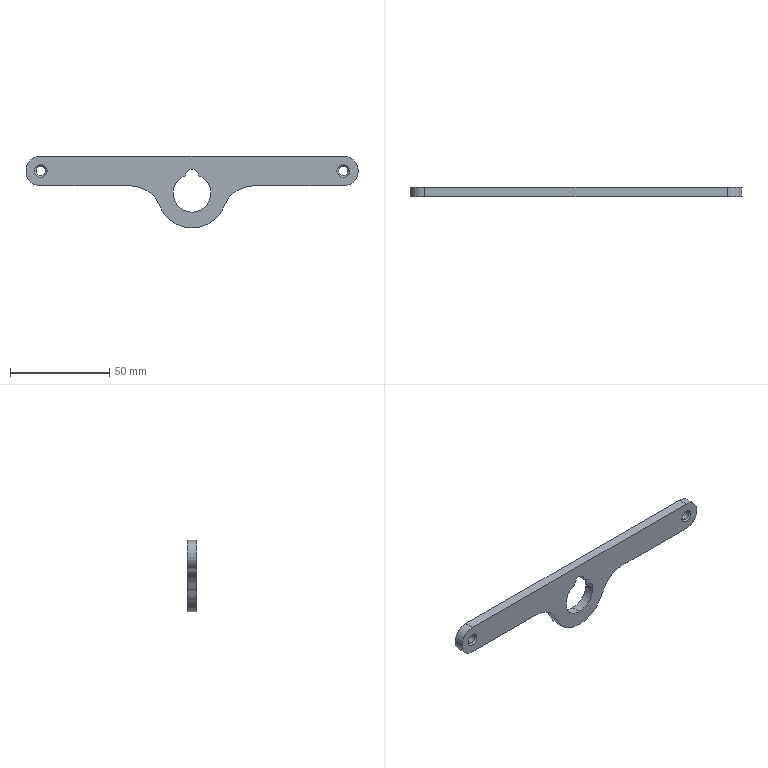Part | SolidWorks | features Chamfer 1, Extrusion 1 | 1 solid | 26 faces | box 167.386 x 4.826 x 36.182 mm | volume 13483 mm3 | cylinder 13 | cone 8 | plane 5 | commonest cylinder face diameters 4.826 x4 14.986 x2 19.025 x2 31.75 x2 34.9 x2 6.35 x1
STEP:
#1=CARTESIAN_POINT('',(-3.,0.065,0.3475));
#2=VERTEX_POINT('',#1);
#3=CARTESIAN_POINT('',(-3.,0.065,0.5375));
#4=VERTEX_POINT('',#3);
#5=CARTESIAN_POINT('',(-3.,0.065,0.4425));
#6=DIRECTION('',(0.,1.,0.));
#7=DIRECTION('',(0.,0.,1.));
#8=AXIS2_PLACEMENT_3D('',#5,#6,#7);
#9=CIRCLE('',#8,0.095);
#10=EDGE_CURVE('',#2,#4,#9,.T.);
#11=ORIENTED_EDGE('',*,*,#10,.F.);
#12=CARTESIAN_POINT('',(-3.,0.095,0.3175));
#13=VERTEX_POINT('',#12);
#14=CARTESIAN_POINT('',(-3.,0.065,0.3475));
#15=DIRECTION('',(0.,0.7071,-0.7071));
#16=VECTOR('',#15,39.37);
#17=LINE('',#14,#16);
#18=EDGE_CURVE('',#2,#13,#17,.T.);
#19=ORIENTED_EDGE('',*,*,#18,.T.);
#20=CARTESIAN_POINT('',(-3.,0.095,0.5675));
#21=VERTEX_POINT('',#20);
#22=CARTESIAN_POINT('',(-3.,0.095,0.4425));
#23=DIRECTION('',(0.,-1.,0.));
#24=DIRECTION('',(0.,0.,1.));
#25=AXIS2_PLACEMENT_3D('',#22,#23,#24);
#26=CIRCLE('',#25,0.125);
#27=EDGE_CURVE('',#21,#13,#26,.T.);
#28=ORIENTED_EDGE('',*,*,#27,.F.);
#29=CARTESIAN_POINT('',(-3.,0.065,0.5375));
#30=DIRECTION('',(0.,0.7071,0.7071));
#31=VECTOR('',#30,39.37);
#32=LINE('',#29,#31);
#33=EDGE_CURVE('',#4,#21,#32,.T.);
#34=ORIENTED_EDGE('',*,*,#33,.F.);
#35=EDGE_LOOP('',(#11,#19,#28,#34));
#36=FACE_OUTER_BOUND('',#35,.T.);
#37=CARTESIAN_POINT('',(-3.,0.065,0.4425));
#38=DIRECTION('',(0.,1.,0.));
#39=DIRECTION('',(0.,0.,1.));
#40=AXIS2_PLACEMENT_3D('',#37,#38,#39);
#41=CONICAL_SURFACE('',#40,0.095,0.7854);
#42=ADVANCED_FACE('',(#36),#41,.F.);
#43=CARTESIAN_POINT('',(-3.,-0.065,0.5375));
#44=VERTEX_POINT('',#43);
#45=CARTESIAN_POINT('',(-3.,-0.065,0.3475));
#46=VERTEX_POINT('',#45);
#47=CARTESIAN_POINT('',(-3.,-0.065,0.4425));
#48=DIRECTION('',(0.,-1.,0.));
#49=DIRECTION('',(0.,0.,1.));
#50=AXIS2_PLACEMENT_3D('',#47,#48,#49);
#51=CIRCLE('',#50,0.095);
#52=EDGE_CURVE('',#44,#46,#51,.T.);
#53=ORIENTED_EDGE('',*,*,#52,.F.);
#54=CARTESIAN_POINT('',(-3.,-0.095,0.5675));
#55=VERTEX_POINT('',#54);
#56=CARTESIAN_POINT('',(-3.,-0.095,0.5675));
#57=DIRECTION('',(0.,-0.7071,0.7071));
#58=VECTOR('',#57,39.37);
#59=LINE('',#56,#58);
#60=EDGE_CURVE('',#44,#55,#59,.T.);
#61=ORIENTED_EDGE('',*,*,#60,.T.);
#62=CARTESIAN_POINT('',(-3.,-0.095,0.3175));
#63=VERTEX_POINT('',#62);
#64=CARTESIAN_POINT('',(-3.,-0.095,0.4425));
#65=DIRECTION('',(0.,1.,0.));
#66=DIRECTION('',(0.,0.,1.));
#67=AXIS2_PLACEMENT_3D('',#64,#65,#66);
#68=CIRCLE('',#67,0.125);
#69=EDGE_CURVE('',#63,#55,#68,.T.);
#70=ORIENTED_EDGE('',*,*,#69,.F.);
#71=CARTESIAN_POINT('',(-3.,-0.095,0.3175));
#72=DIRECTION('',(0.,-0.7071,-0.7071));
#73=VECTOR('',#72,39.37);
#74=LINE('',#71,#73);
#75=EDGE_CURVE('',#46,#63,#74,.T.);
#76=ORIENTED_EDGE('',*,*,#75,.F.);
#77=EDGE_LOOP('',(#53,#61,#70,#76));
#78=FACE_OUTER_BOUND('',#77,.T.);
#79=CARTESIAN_POINT('',(-3.,-0.095,0.4425));
#80=DIRECTION('',(0.,-1.,0.));
#81=DIRECTION('',(0.,0.,-1.));
#82=AXIS2_PLACEMENT_3D('',#79,#80,#81);
#83=CONICAL_SURFACE('',#82,0.125,0.7854);
#84=ADVANCED_FACE('',(#78),#83,.F.);
#85=CARTESIAN_POINT('',(3.,0.065,0.3475));
#86=VERTEX_POINT('',#85);
#87=CARTESIAN_POINT('',(3.,0.065,0.5375));
#88=VERTEX_POINT('',#87);
#89=CARTESIAN_POINT('',(3.,0.065,0.4425));
#90=DIRECTION('',(0.,1.,0.));
#91=DIRECTION('',(0.,0.,1.));
#92=AXIS2_PLACEMENT_3D('',#89,#90,#91);
#93=CIRCLE('',#92,0.095);
#94=EDGE_CURVE('',#86,#88,#93,.T.);
#95=ORIENTED_EDGE('',*,*,#94,.F.);
#96=CARTESIAN_POINT('',(3.,0.095,0.3175));
#97=VERTEX_POINT('',#96);
#98=CARTESIAN_POINT('',(3.,0.065,0.3475));
#99=DIRECTION('',(0.,0.7071,-0.7071));
#100=VECTOR('',#99,39.37);
#101=LINE('',#98,#100);
#102=EDGE_CURVE('',#86,#97,#101,.T.);
#103=ORIENTED_EDGE('',*,*,#102,.T.);
#104=CARTESIAN_POINT('',(3.,0.095,0.5675));
#105=VERTEX_POINT('',#104);
#106=CARTESIAN_POINT('',(3.,0.095,0.4425));
#107=DIRECTION('',(0.,-1.,0.));
#108=DIRECTION('',(0.,0.,1.));
#109=AXIS2_PLACEMENT_3D('',#106,#107,#108);
#110=CIRCLE('',#109,0.125);
#111=EDGE_CURVE('',#105,#97,#110,.T.);
#112=ORIENTED_EDGE('',*,*,#111,.F.);
#113=CARTESIAN_POINT('',(3.,0.065,0.5375));
#114=DIRECTION('',(0.,0.7071,0.7071));
#115=VECTOR('',#114,39.37);
#116=LINE('',#113,#115);
#117=EDGE_CURVE('',#88,#105,#116,.T.);
#118=ORIENTED_EDGE('',*,*,#117,.F.);
#119=EDGE_LOOP('',(#95,#103,#112,#118));
#120=FACE_OUTER_BOUND('',#119,.T.);
#121=CARTESIAN_POINT('',(3.,0.065,0.4425));
#122=DIRECTION('',(0.,1.,0.));
#123=DIRECTION('',(0.,0.,1.));
#124=AXIS2_PLACEMENT_3D('',#121,#122,#123);
#125=CONICAL_SURFACE('',#124,0.095,0.7854);
#126=ADVANCED_FACE('',(#120),#125,.F.);
#127=CARTESIAN_POINT('',(3.,-0.065,0.5375));
#128=VERTEX_POINT('',#127);
#129=CARTESIAN_POINT('',(3.,-0.065,0.3475));
#130=VERTEX_POINT('',#129);
#131=CARTESIAN_POINT('',(3.,-0.065,0.4425));
#132=DIRECTION('',(0.,-1.,0.));
#133=DIRECTION('',(0.,0.,1.));
#134=AXIS2_PLACEMENT_3D('',#131,#132,#133);
#135=CIRCLE('',#134,0.095);
#136=EDGE_CURVE('',#128,#130,#135,.T.);
#137=ORIENTED_EDGE('',*,*,#136,.F.);
#138=CARTESIAN_POINT('',(3.,-0.095,0.5675));
#139=VERTEX_POINT('',#138);
#140=CARTESIAN_POINT('',(3.,-0.095,0.5675));
#141=DIRECTION('',(0.,-0.7071,0.7071));
#142=VECTOR('',#141,39.37);
#143=LINE('',#140,#142);
#144=EDGE_CURVE('',#128,#139,#143,.T.);
#145=ORIENTED_EDGE('',*,*,#144,.T.);
#146=CARTESIAN_POINT('',(3.,-0.095,0.3175));
#147=VERTEX_POINT('',#146);
#148=CARTESIAN_POINT('',(3.,-0.095,0.4425));
#149=DIRECTION('',(0.,1.,0.));
#150=DIRECTION('',(0.,0.,1.));
#151=AXIS2_PLACEMENT_3D('',#148,#149,#150);
#152=CIRCLE('',#151,0.125);
#153=EDGE_CURVE('',#147,#139,#152,.T.);
#154=ORIENTED_EDGE('',*,*,#153,.F.);
#155=CARTESIAN_POINT('',(3.,-0.095,0.3175));
#156=DIRECTION('',(0.,-0.7071,-0.7071));
#157=VECTOR('',#156,39.37);
#158=LINE('',#155,#157);
#159=EDGE_CURVE('',#130,#147,#158,.T.);
#160=ORIENTED_EDGE('',*,*,#159,.F.);
#161=EDGE_LOOP('',(#137,#145,#154,#160));
#162=FACE_OUTER_BOUND('',#161,.T.);
#163=CARTESIAN_POINT('',(3.,-0.095,0.4425));
#164=DIRECTION('',(0.,-1.,0.));
#165=DIRECTION('',(0.,0.,-1.));
#166=AXIS2_PLACEMENT_3D('',#163,#164,#165);
#167=CONICAL_SURFACE('',#166,0.125,0.7854);
#168=ADVANCED_FACE('',(#162),#167,.F.);
#169=CARTESIAN_POINT('',(0.125,0.095,0.353));
#170=VERTEX_POINT('',#169);
#171=CARTESIAN_POINT('',(0.,0.095,-0.3745));
#172=VERTEX_POINT('',#171);
#173=CARTESIAN_POINT('',(0.,0.095,0.));
#174=DIRECTION('',(0.,1.,0.));
#175=DIRECTION('',(0.,0.,1.));
#176=AXIS2_PLACEMENT_3D('',#173,#174,#175);
#177=CIRCLE('',#176,0.3745);
#178=EDGE_CURVE('',#170,#172,#177,.T.);
#179=ORIENTED_EDGE('',*,*,#178,.T.);
#180=CARTESIAN_POINT('',(0.,-0.095,-0.3745));
#181=VERTEX_POINT('',#180);
#182=CARTESIAN_POINT('',(0.,0.095,-0.3745));
#183=DIRECTION('',(0.,-1.,0.));
#184=VECTOR('',#183,39.37);
#185=LINE('',#182,#184);
#186=EDGE_CURVE('',#172,#181,#185,.T.);
#187=ORIENTED_EDGE('',*,*,#186,.T.);
#188=CARTESIAN_POINT('',(0.125,-0.095,0.353));
#189=VERTEX_POINT('',#188);
#190=CARTESIAN_POINT('',(0.,-0.095,0.));
#191=DIRECTION('',(0.,1.,0.));
#192=DIRECTION('',(0.,0.,1.));
#193=AXIS2_PLACEMENT_3D('',#190,#191,#192);
#194=CIRCLE('',#193,0.3745);
#195=EDGE_CURVE('',#189,#181,#194,.T.);
#196=ORIENTED_EDGE('',*,*,#195,.F.);
#197=CARTESIAN_POINT('',(0.125,0.095,0.353));
#198=DIRECTION('',(0.,-1.,0.));
#199=VECTOR('',#198,39.37);
#200=LINE('',#197,#199);
#201=EDGE_CURVE('',#170,#189,#200,.T.);
#202=ORIENTED_EDGE('',*,*,#201,.F.);
#203=EDGE_LOOP('',(#179,#187,#196,#202));
#204=FACE_OUTER_BOUND('',#203,.T.);
#205=CARTESIAN_POINT('',(0.,0.095,0.));
#206=DIRECTION('',(0.,-1.,0.));
#207=DIRECTION('',(0.,0.,-1.));
#208=AXIS2_PLACEMENT_3D('',#205,#206,#207);
#209=CYLINDRICAL_SURFACE('',#208,0.3745);
#210=ADVANCED_FACE('',(#204),#209,.F.);
#211=ORIENTED_EDGE('',*,*,#10,.T.);
#212=CARTESIAN_POINT('',(-3.,0.095,0.5375));
#213=DIRECTION('',(0.,-1.,0.));
#214=VECTOR('',#213,39.37);
#215=LINE('',#212,#214);
#216=EDGE_CURVE('',#4,#44,#215,.T.);
#217=ORIENTED_EDGE('',*,*,#216,.T.);
#218=ORIENTED_EDGE('',*,*,#52,.T.);
#219=CARTESIAN_POINT('',(-3.,0.095,0.3475));
#220=DIRECTION('',(0.,-1.,0.));
#221=VECTOR('',#220,39.37);
#222=LINE('',#219,#221);
#223=EDGE_CURVE('',#2,#46,#222,.T.);
#224=ORIENTED_EDGE('',*,*,#223,.F.);
#225=EDGE_LOOP('',(#211,#217,#218,#224));
#226=FACE_OUTER_BOUND('',#225,.T.);
#227=CARTESIAN_POINT('',(-3.,0.095,0.4425));
#228=DIRECTION('',(0.,-1.,0.));
#229=DIRECTION('',(0.,0.,-1.));
#230=AXIS2_PLACEMENT_3D('',#227,#228,#229);
#231=CYLINDRICAL_SURFACE('',#230,0.095);
#232=ADVANCED_FACE('',(#226),#231,.F.);
#233=ORIENTED_EDGE('',*,*,#94,.T.);
#234=CARTESIAN_POINT('',(3.,0.095,0.5375));
#235=DIRECTION('',(0.,-1.,0.));
#236=VECTOR('',#235,39.37);
#237=LINE('',#234,#236);
#238=EDGE_CURVE('',#88,#128,#237,.T.);
#239=ORIENTED_EDGE('',*,*,#238,.T.);
#240=ORIENTED_EDGE('',*,*,#136,.T.);
#241=CARTESIAN_POINT('',(3.,0.095,0.3475));
#242=DIRECTION('',(0.,-1.,0.));
#243=VECTOR('',#242,39.37);
#244=LINE('',#241,#243);
#245=EDGE_CURVE('',#86,#130,#244,.T.);
#246=ORIENTED_EDGE('',*,*,#245,.F.);
#247=EDGE_LOOP('',(#233,#239,#240,#246));
#248=FACE_OUTER_BOUND('',#247,.T.);
#249=CARTESIAN_POINT('',(3.,0.095,0.4425));
#250=DIRECTION('',(0.,-1.,0.));
#251=DIRECTION('',(0.,0.,-1.));
#252=AXIS2_PLACEMENT_3D('',#249,#250,#251);
#253=CYLINDRICAL_SURFACE('',#252,0.095);
#254=ADVANCED_FACE('',(#248),#253,.F.);
#255=CARTESIAN_POINT('',(0.,0.095,-0.687));
#256=VERTEX_POINT('',#255);
#257=CARTESIAN_POINT('',(-0.6399,0.095,-0.25));
#258=VERTEX_POINT('',#257);
#259=CARTESIAN_POINT('',(0.,0.095,0.));
#260=DIRECTION('',(0.,1.,0.));
#261=DIRECTION('',(0.,0.,1.));
#262=AXIS2_PLACEMENT_3D('',#259,#260,#261);
#263=CIRCLE('',#262,0.687);
#264=EDGE_CURVE('',#256,#258,#263,.T.);
#265=ORIENTED_EDGE('',*,*,#264,.F.);
#266=CARTESIAN_POINT('',(0.,-0.095,-0.687));
#267=VERTEX_POINT('',#266);
#268=CARTESIAN_POINT('',(0.,0.095,-0.687));
#269=DIRECTION('',(0.,-1.,0.));
#270=VECTOR('',#269,39.37);
#271=LINE('',#268,#270);
#272=EDGE_CURVE('',#256,#267,#271,.T.);
#273=ORIENTED_EDGE('',*,*,#272,.T.);
#274=CARTESIAN_POINT('',(-0.6399,-0.095,-0.25));
#275=VERTEX_POINT('',#274);
#276=CARTESIAN_POINT('',(0.,-0.095,0.));
#277=DIRECTION('',(0.,1.,0.));
#278=DIRECTION('',(0.,0.,1.));
#279=AXIS2_PLACEMENT_3D('',#276,#277,#278);
#280=CIRCLE('',#279,0.687);
#281=EDGE_CURVE('',#267,#275,#280,.T.);
#282=ORIENTED_EDGE('',*,*,#281,.T.);
#283=CARTESIAN_POINT('',(-0.6399,0.095,-0.25));
#284=DIRECTION('',(0.,-1.,0.));
#285=VECTOR('',#284,39.37);
#286=LINE('',#283,#285);
#287=EDGE_CURVE('',#258,#275,#286,.T.);
#288=ORIENTED_EDGE('',*,*,#287,.F.);
#289=EDGE_LOOP('',(#265,#273,#282,#288));
#290=FACE_OUTER_BOUND('',#289,.T.);
#291=CARTESIAN_POINT('',(0.,0.095,0.));
#292=DIRECTION('',(0.,-1.,0.));
#293=DIRECTION('',(0.,0.,-1.));
#294=AXIS2_PLACEMENT_3D('',#291,#292,#293);
#295=CYLINDRICAL_SURFACE('',#294,0.687);
#296=ADVANCED_FACE('',(#290),#295,.T.);
#297=ORIENTED_EDGE('',*,*,#111,.T.);
#298=CARTESIAN_POINT('',(3.,0.095,0.4425));
#299=DIRECTION('',(0.,-1.,0.));
#300=DIRECTION('',(0.,0.,1.));
#301=AXIS2_PLACEMENT_3D('',#298,#299,#300);
#302=CIRCLE('',#301,0.125);
#303=EDGE_CURVE('',#97,#105,#302,.T.);
#304=ORIENTED_EDGE('',*,*,#303,.T.);
#305=EDGE_LOOP('',(#297,#304));
#306=FACE_BOUND('',#305,.T.);
#307=ORIENTED_EDGE('',*,*,#27,.T.);
#308=CARTESIAN_POINT('',(-3.,0.095,0.4425));
#309=DIRECTION('',(0.,-1.,0.));
#310=DIRECTION('',(0.,0.,1.));
#311=AXIS2_PLACEMENT_3D('',#308,#309,#310);
#312=CIRCLE('',#311,0.125);
#313=EDGE_CURVE('',#13,#21,#312,.T.);
#314=ORIENTED_EDGE('',*,*,#313,.T.);
#315=EDGE_LOOP('',(#307,#314));
#316=FACE_BOUND('',#315,.T.);
#317=CARTESIAN_POINT('',(-1.222,0.095,0.1475));
#318=VERTEX_POINT('',#317);
#319=CARTESIAN_POINT('',(-1.222,0.095,-0.4775));
#320=DIRECTION('',(0.,-1.,0.));
#321=DIRECTION('',(0.,0.,1.));
#322=AXIS2_PLACEMENT_3D('',#319,#320,#321);
#323=CIRCLE('',#322,0.625);
#324=EDGE_CURVE('',#258,#318,#323,.T.);
#325=ORIENTED_EDGE('',*,*,#324,.T.);
#326=CARTESIAN_POINT('',(-3.,0.095,0.1475));
#327=VERTEX_POINT('',#326);
#328=CARTESIAN_POINT('',(-3.,0.095,0.1475));
#329=DIRECTION('',(-1.,0.,0.));
#330=VECTOR('',#329,39.37);
#331=LINE('',#328,#330);
#332=EDGE_CURVE('',#318,#327,#331,.T.);
#333=ORIENTED_EDGE('',*,*,#332,.T.);
#334=CARTESIAN_POINT('',(-3.,0.095,0.7375));
#335=VERTEX_POINT('',#334);
#336=CARTESIAN_POINT('',(-3.,0.095,0.4425));
#337=DIRECTION('',(0.,1.,0.));
#338=DIRECTION('',(0.,0.,1.));
#339=AXIS2_PLACEMENT_3D('',#336,#337,#338);
#340=CIRCLE('',#339,0.295);
#341=EDGE_CURVE('',#327,#335,#340,.T.);
#342=ORIENTED_EDGE('',*,*,#341,.T.);
#343=CARTESIAN_POINT('',(3.,0.095,0.7375));
#344=VERTEX_POINT('',#343);
#345=CARTESIAN_POINT('',(-3.,0.095,0.7375));
#346=DIRECTION('',(1.,0.,0.));
#347=VECTOR('',#346,39.37);
#348=LINE('',#345,#347);
#349=EDGE_CURVE('',#335,#344,#348,.T.);
#350=ORIENTED_EDGE('',*,*,#349,.T.);
#351=CARTESIAN_POINT('',(3.,0.095,0.1475));
#352=VERTEX_POINT('',#351);
#353=CARTESIAN_POINT('',(3.,0.095,0.4425));
#354=DIRECTION('',(0.,1.,0.));
#355=DIRECTION('',(0.,0.,1.));
#356=AXIS2_PLACEMENT_3D('',#353,#354,#355);
#357=CIRCLE('',#356,0.295);
#358=EDGE_CURVE('',#344,#352,#357,.T.);
#359=ORIENTED_EDGE('',*,*,#358,.T.);
#360=CARTESIAN_POINT('',(1.222,0.095,0.1475));
#361=VERTEX_POINT('',#360);
#362=CARTESIAN_POINT('',(1.222,0.095,0.1475));
#363=DIRECTION('',(-1.,0.,0.));
#364=VECTOR('',#363,39.37);
#365=LINE('',#362,#364);
#366=EDGE_CURVE('',#352,#361,#365,.T.);
#367=ORIENTED_EDGE('',*,*,#366,.T.);
#368=CARTESIAN_POINT('',(0.6399,0.095,-0.25));
#369=VERTEX_POINT('',#368);
#370=CARTESIAN_POINT('',(1.222,0.095,-0.4775));
#371=DIRECTION('',(0.,-1.,0.));
#372=DIRECTION('',(0.,0.,-1.));
#373=AXIS2_PLACEMENT_3D('',#370,#371,#372);
#374=CIRCLE('',#373,0.625);
#375=EDGE_CURVE('',#361,#369,#374,.T.);
#376=ORIENTED_EDGE('',*,*,#375,.T.);
#377=CARTESIAN_POINT('',(0.,0.095,0.));
#378=DIRECTION('',(0.,1.,0.));
#379=DIRECTION('',(0.,0.,1.));
#380=AXIS2_PLACEMENT_3D('',#377,#378,#379);
#381=CIRCLE('',#380,0.687);
#382=EDGE_CURVE('',#369,#256,#381,.T.);
#383=ORIENTED_EDGE('',*,*,#382,.T.);
#384=ORIENTED_EDGE('',*,*,#264,.T.);
#385=EDGE_LOOP('',(#325,#333,#342,#350,#359,#367,#376,#383,#384));
#386=FACE_OUTER_BOUND('',#385,.T.);
#387=ORIENTED_EDGE('',*,*,#178,.F.);
#388=CARTESIAN_POINT('',(-0.125,0.095,0.353));
#389=VERTEX_POINT('',#388);
#390=CARTESIAN_POINT('',(0.,0.095,0.3525));
#391=DIRECTION('',(0.,1.,0.));
#392=DIRECTION('',(0.,0.,1.));
#393=AXIS2_PLACEMENT_3D('',#390,#391,#392);
#394=CIRCLE('',#393,0.125);
#395=EDGE_CURVE('',#389,#170,#394,.T.);
#396=ORIENTED_EDGE('',*,*,#395,.F.);
#397=CARTESIAN_POINT('',(0.,0.095,0.));
#398=DIRECTION('',(0.,1.,0.));
#399=DIRECTION('',(0.,0.,1.));
#400=AXIS2_PLACEMENT_3D('',#397,#398,#399);
#401=CIRCLE('',#400,0.3745);
#402=EDGE_CURVE('',#172,#389,#401,.T.);
#403=ORIENTED_EDGE('',*,*,#402,.F.);
#404=EDGE_LOOP('',(#387,#396,#403));
#405=FACE_BOUND('',#404,.T.);
#406=CARTESIAN_POINT('',(-1.222,0.095,-0.4775));
#407=DIRECTION('',(0.,1.,0.));
#408=DIRECTION('',(0.,0.,1.));
#409=AXIS2_PLACEMENT_3D('',#406,#407,#408);
#410=PLANE('',#409);
#411=ADVANCED_FACE('',(#306,#316,#386,#405),#410,.T.);
#412=ORIENTED_EDGE('',*,*,#153,.T.);
#413=CARTESIAN_POINT('',(3.,-0.095,0.4425));
#414=DIRECTION('',(0.,1.,0.));
#415=DIRECTION('',(0.,0.,1.));
#416=AXIS2_PLACEMENT_3D('',#413,#414,#415);
#417=CIRCLE('',#416,0.125);
#418=EDGE_CURVE('',#139,#147,#417,.T.);
#419=ORIENTED_EDGE('',*,*,#418,.T.);
#420=EDGE_LOOP('',(#412,#419));
#421=FACE_BOUND('',#420,.T.);
#422=ORIENTED_EDGE('',*,*,#69,.T.);
#423=CARTESIAN_POINT('',(-3.,-0.095,0.4425));
#424=DIRECTION('',(0.,1.,0.));
#425=DIRECTION('',(0.,0.,1.));
#426=AXIS2_PLACEMENT_3D('',#423,#424,#425);
#427=CIRCLE('',#426,0.125);
#428=EDGE_CURVE('',#55,#63,#427,.T.);
#429=ORIENTED_EDGE('',*,*,#428,.T.);
#430=EDGE_LOOP('',(#422,#429));
#431=FACE_BOUND('',#430,.T.);
#432=CARTESIAN_POINT('',(-1.222,-0.095,0.1475));
#433=VERTEX_POINT('',#432);
#434=CARTESIAN_POINT('',(-1.222,-0.095,-0.4775));
#435=DIRECTION('',(0.,-1.,0.));
#436=DIRECTION('',(0.,0.,1.));
#437=AXIS2_PLACEMENT_3D('',#434,#435,#436);
#438=CIRCLE('',#437,0.625);
#439=EDGE_CURVE('',#275,#433,#438,.T.);
#440=ORIENTED_EDGE('',*,*,#439,.F.);
#441=ORIENTED_EDGE('',*,*,#281,.F.);
#442=CARTESIAN_POINT('',(0.6399,-0.095,-0.25));
#443=VERTEX_POINT('',#442);
#444=CARTESIAN_POINT('',(0.,-0.095,0.));
#445=DIRECTION('',(0.,1.,0.));
#446=DIRECTION('',(0.,0.,1.));
#447=AXIS2_PLACEMENT_3D('',#444,#445,#446);
#448=CIRCLE('',#447,0.687);
#449=EDGE_CURVE('',#443,#267,#448,.T.);
#450=ORIENTED_EDGE('',*,*,#449,.F.);
#451=CARTESIAN_POINT('',(1.222,-0.095,0.1475));
#452=VERTEX_POINT('',#451);
#453=CARTESIAN_POINT('',(1.222,-0.095,-0.4775));
#454=DIRECTION('',(0.,-1.,0.));
#455=DIRECTION('',(0.,0.,-1.));
#456=AXIS2_PLACEMENT_3D('',#453,#454,#455);
#457=CIRCLE('',#456,0.625);
#458=EDGE_CURVE('',#452,#443,#457,.T.);
#459=ORIENTED_EDGE('',*,*,#458,.F.);
#460=CARTESIAN_POINT('',(3.,-0.095,0.1475));
#461=VERTEX_POINT('',#460);
#462=CARTESIAN_POINT('',(1.222,-0.095,0.1475));
#463=DIRECTION('',(-1.,0.,0.));
#464=VECTOR('',#463,39.37);
#465=LINE('',#462,#464);
#466=EDGE_CURVE('',#461,#452,#465,.T.);
#467=ORIENTED_EDGE('',*,*,#466,.F.);
#468=CARTESIAN_POINT('',(3.,-0.095,0.7375));
#469=VERTEX_POINT('',#468);
#470=CARTESIAN_POINT('',(3.,-0.095,0.4425));
#471=DIRECTION('',(0.,1.,0.));
#472=DIRECTION('',(0.,0.,1.));
#473=AXIS2_PLACEMENT_3D('',#470,#471,#472);
#474=CIRCLE('',#473,0.295);
#475=EDGE_CURVE('',#469,#461,#474,.T.);
#476=ORIENTED_EDGE('',*,*,#475,.F.);
#477=CARTESIAN_POINT('',(-3.,-0.095,0.7375));
#478=VERTEX_POINT('',#477);
#479=CARTESIAN_POINT('',(-3.,-0.095,0.7375));
#480=DIRECTION('',(1.,0.,0.));
#481=VECTOR('',#480,39.37);
#482=LINE('',#479,#481);
#483=EDGE_CURVE('',#478,#469,#482,.T.);
#484=ORIENTED_EDGE('',*,*,#483,.F.);
#485=CARTESIAN_POINT('',(-3.,-0.095,0.1475));
#486=VERTEX_POINT('',#485);
#487=CARTESIAN_POINT('',(-3.,-0.095,0.4425));
#488=DIRECTION('',(0.,1.,0.));
#489=DIRECTION('',(0.,0.,1.));
#490=AXIS2_PLACEMENT_3D('',#487,#488,#489);
#491=CIRCLE('',#490,0.295);
#492=EDGE_CURVE('',#486,#478,#491,.T.);
#493=ORIENTED_EDGE('',*,*,#492,.F.);
#494=CARTESIAN_POINT('',(-3.,-0.095,0.1475));
#495=DIRECTION('',(-1.,0.,0.));
#496=VECTOR('',#495,39.37);
#497=LINE('',#494,#496);
#498=EDGE_CURVE('',#433,#486,#497,.T.);
#499=ORIENTED_EDGE('',*,*,#498,.F.);
#500=EDGE_LOOP('',(#440,#441,#450,#459,#467,#476,#484,#493,#499));
#501=FACE_OUTER_BOUND('',#500,.T.);
#502=CARTESIAN_POINT('',(-0.125,-0.095,0.353));
#503=VERTEX_POINT('',#502);
#504=CARTESIAN_POINT('',(0.,-0.095,0.3525));
#505=DIRECTION('',(0.,1.,0.));
#506=DIRECTION('',(0.,0.,1.));
#507=AXIS2_PLACEMENT_3D('',#504,#505,#506);
#508=CIRCLE('',#507,0.125);
#509=EDGE_CURVE('',#503,#189,#508,.T.);
#510=ORIENTED_EDGE('',*,*,#509,.T.);
#511=ORIENTED_EDGE('',*,*,#195,.T.);
#512=CARTESIAN_POINT('',(0.,-0.095,0.));
#513=DIRECTION('',(0.,1.,0.));
#514=DIRECTION('',(0.,0.,1.));
#515=AXIS2_PLACEMENT_3D('',#512,#513,#514);
#516=CIRCLE('',#515,0.3745);
#517=EDGE_CURVE('',#181,#503,#516,.T.);
#518=ORIENTED_EDGE('',*,*,#517,.T.);
#519=EDGE_LOOP('',(#510,#511,#518));
#520=FACE_BOUND('',#519,.T.);
#521=CARTESIAN_POINT('',(-1.222,-0.095,-0.4775));
#522=DIRECTION('',(0.,1.,0.));
#523=DIRECTION('',(0.,0.,1.));
#524=AXIS2_PLACEMENT_3D('',#521,#522,#523);
#525=PLANE('',#524);
#526=ADVANCED_FACE('',(#421,#431,#501,#520),#525,.F.);
#527=ORIENTED_EDGE('',*,*,#439,.T.);
#528=CARTESIAN_POINT('',(-1.222,0.095,0.1475));
#529=DIRECTION('',(0.,-1.,0.));
#530=VECTOR('',#529,39.37);
#531=LINE('',#528,#530);
#532=EDGE_CURVE('',#318,#433,#531,.T.);
#533=ORIENTED_EDGE('',*,*,#532,.F.);
#534=ORIENTED_EDGE('',*,*,#324,.F.);
#535=ORIENTED_EDGE('',*,*,#287,.T.);
#536=EDGE_LOOP('',(#527,#533,#534,#535));
#537=FACE_OUTER_BOUND('',#536,.T.);
#538=CARTESIAN_POINT('',(-1.222,0.095,-0.4775));
#539=DIRECTION('',(0.,-1.,0.));
#540=DIRECTION('',(0.,0.,-1.));
#541=AXIS2_PLACEMENT_3D('',#538,#539,#540);
#542=CYLINDRICAL_SURFACE('',#541,0.625);
#543=ADVANCED_FACE('',(#537),#542,.F.);
#544=ORIENTED_EDGE('',*,*,#498,.T.);
#545=CARTESIAN_POINT('',(-3.,0.095,0.1475));
#546=DIRECTION('',(0.,-1.,0.));
#547=VECTOR('',#546,39.37);
#548=LINE('',#545,#547);
#549=EDGE_CURVE('',#327,#486,#548,.T.);
#550=ORIENTED_EDGE('',*,*,#549,.F.);
#551=ORIENTED_EDGE('',*,*,#332,.F.);
#552=ORIENTED_EDGE('',*,*,#532,.T.);
#553=EDGE_LOOP('',(#544,#550,#551,#552));
#554=FACE_OUTER_BOUND('',#553,.T.);
#555=CARTESIAN_POINT('',(-3.,0.095,0.1475));
#556=DIRECTION('',(0.,0.,1.));
#557=DIRECTION('',(1.,0.,0.));
#558=AXIS2_PLACEMENT_3D('',#555,#556,#557);
#559=PLANE('',#558);
#560=ADVANCED_FACE('',(#554),#559,.F.);
#561=ORIENTED_EDGE('',*,*,#492,.T.);
#562=CARTESIAN_POINT('',(-3.,0.095,0.7375));
#563=DIRECTION('',(0.,-1.,0.));
#564=VECTOR('',#563,39.37);
#565=LINE('',#562,#564);
#566=EDGE_CURVE('',#335,#478,#565,.T.);
#567=ORIENTED_EDGE('',*,*,#566,.F.);
#568=ORIENTED_EDGE('',*,*,#341,.F.);
#569=ORIENTED_EDGE('',*,*,#549,.T.);
#570=EDGE_LOOP('',(#561,#567,#568,#569));
#571=FACE_OUTER_BOUND('',#570,.T.);
#572=CARTESIAN_POINT('',(-3.,0.095,0.4425));
#573=DIRECTION('',(0.,-1.,0.));
#574=DIRECTION('',(0.,0.,-1.));
#575=AXIS2_PLACEMENT_3D('',#572,#573,#574);
#576=CYLINDRICAL_SURFACE('',#575,0.295);
#577=ADVANCED_FACE('',(#571),#576,.T.);
#578=ORIENTED_EDGE('',*,*,#483,.T.);
#579=CARTESIAN_POINT('',(3.,0.095,0.7375));
#580=DIRECTION('',(0.,-1.,0.));
#581=VECTOR('',#580,39.37);
#582=LINE('',#579,#581);
#583=EDGE_CURVE('',#344,#469,#582,.T.);
#584=ORIENTED_EDGE('',*,*,#583,.F.);
#585=ORIENTED_EDGE('',*,*,#349,.F.);
#586=ORIENTED_EDGE('',*,*,#566,.T.);
#587=EDGE_LOOP('',(#578,#584,#585,#586));
#588=FACE_OUTER_BOUND('',#587,.T.);
#589=CARTESIAN_POINT('',(-3.,0.095,0.7375));
#590=DIRECTION('',(0.,0.,-1.));
#591=DIRECTION('',(-1.,0.,0.));
#592=AXIS2_PLACEMENT_3D('',#589,#590,#591);
#593=PLANE('',#592);
#594=ADVANCED_FACE('',(#588),#593,.F.);
#595=ORIENTED_EDGE('',*,*,#475,.T.);
#596=CARTESIAN_POINT('',(3.,0.095,0.1475));
#597=DIRECTION('',(0.,-1.,0.));
#598=VECTOR('',#597,39.37);
#599=LINE('',#596,#598);
#600=EDGE_CURVE('',#352,#461,#599,.T.);
#601=ORIENTED_EDGE('',*,*,#600,.F.);
#602=ORIENTED_EDGE('',*,*,#358,.F.);
#603=ORIENTED_EDGE('',*,*,#583,.T.);
#604=EDGE_LOOP('',(#595,#601,#602,#603));
#605=FACE_OUTER_BOUND('',#604,.T.);
#606=CARTESIAN_POINT('',(3.,0.095,0.4425));
#607=DIRECTION('',(0.,-1.,0.));
#608=DIRECTION('',(0.,0.,-1.));
#609=AXIS2_PLACEMENT_3D('',#606,#607,#608);
#610=CYLINDRICAL_SURFACE('',#609,0.295);
#611=ADVANCED_FACE('',(#605),#610,.T.);
#612=ORIENTED_EDGE('',*,*,#466,.T.);
#613=CARTESIAN_POINT('',(1.222,0.095,0.1475));
#614=DIRECTION('',(0.,-1.,0.));
#615=VECTOR('',#614,39.37);
#616=LINE('',#613,#615);
#617=EDGE_CURVE('',#361,#452,#616,.T.);
#618=ORIENTED_EDGE('',*,*,#617,.F.);
#619=ORIENTED_EDGE('',*,*,#366,.F.);
#620=ORIENTED_EDGE('',*,*,#600,.T.);
#621=EDGE_LOOP('',(#612,#618,#619,#620));
#622=FACE_OUTER_BOUND('',#621,.T.);
#623=CARTESIAN_POINT('',(1.222,0.095,0.1475));
#624=DIRECTION('',(0.,0.,1.));
#625=DIRECTION('',(1.,0.,0.));
#626=AXIS2_PLACEMENT_3D('',#623,#624,#625);
#627=PLANE('',#626);
#628=ADVANCED_FACE('',(#622),#627,.F.);
#629=ORIENTED_EDGE('',*,*,#458,.T.);
#630=CARTESIAN_POINT('',(0.6399,0.095,-0.25));
#631=DIRECTION('',(0.,-1.,0.));
#632=VECTOR('',#631,39.37);
#633=LINE('',#630,#632);
#634=EDGE_CURVE('',#369,#443,#633,.T.);
#635=ORIENTED_EDGE('',*,*,#634,.F.);
#636=ORIENTED_EDGE('',*,*,#375,.F.);
#637=ORIENTED_EDGE('',*,*,#617,.T.);
#638=EDGE_LOOP('',(#629,#635,#636,#637));
#639=FACE_OUTER_BOUND('',#638,.T.);
#640=CARTESIAN_POINT('',(1.222,0.095,-0.4775));
#641=DIRECTION('',(0.,-1.,0.));
#642=DIRECTION('',(0.,0.,-1.));
#643=AXIS2_PLACEMENT_3D('',#640,#641,#642);
#644=CYLINDRICAL_SURFACE('',#643,0.625);
#645=ADVANCED_FACE('',(#639),#644,.F.);
#646=ORIENTED_EDGE('',*,*,#272,.F.);
#647=ORIENTED_EDGE('',*,*,#382,.F.);
#648=ORIENTED_EDGE('',*,*,#634,.T.);
#649=ORIENTED_EDGE('',*,*,#449,.T.);
#650=EDGE_LOOP('',(#646,#647,#648,#649));
#651=FACE_OUTER_BOUND('',#650,.T.);
#652=CARTESIAN_POINT('',(0.,0.095,0.));
#653=DIRECTION('',(0.,-1.,0.));
#654=DIRECTION('',(0.,0.,-1.));
#655=AXIS2_PLACEMENT_3D('',#652,#653,#654);
#656=CYLINDRICAL_SURFACE('',#655,0.687);
#657=ADVANCED_FACE('',(#651),#656,.T.);
#658=ORIENTED_EDGE('',*,*,#238,.F.);
#659=CARTESIAN_POINT('',(3.,0.065,0.4425));
#660=DIRECTION('',(0.,1.,0.));
#661=DIRECTION('',(0.,0.,1.));
#662=AXIS2_PLACEMENT_3D('',#659,#660,#661);
#663=CIRCLE('',#662,0.095);
#664=EDGE_CURVE('',#88,#86,#663,.T.);
#665=ORIENTED_EDGE('',*,*,#664,.T.);
#666=ORIENTED_EDGE('',*,*,#245,.T.);
#667=CARTESIAN_POINT('',(3.,-0.065,0.4425));
#668=DIRECTION('',(0.,-1.,0.));
#669=DIRECTION('',(0.,0.,1.));
#670=AXIS2_PLACEMENT_3D('',#667,#668,#669);
#671=CIRCLE('',#670,0.095);
#672=EDGE_CURVE('',#130,#128,#671,.T.);
#673=ORIENTED_EDGE('',*,*,#672,.T.);
#674=EDGE_LOOP('',(#658,#665,#666,#673));
#675=FACE_OUTER_BOUND('',#674,.T.);
#676=CARTESIAN_POINT('',(3.,0.095,0.4425));
#677=DIRECTION('',(0.,-1.,0.));
#678=DIRECTION('',(0.,0.,-1.));
#679=AXIS2_PLACEMENT_3D('',#676,#677,#678);
#680=CYLINDRICAL_SURFACE('',#679,0.095);
#681=ADVANCED_FACE('',(#675),#680,.F.);
#682=ORIENTED_EDGE('',*,*,#216,.F.);
#683=CARTESIAN_POINT('',(-3.,0.065,0.4425));
#684=DIRECTION('',(0.,1.,0.));
#685=DIRECTION('',(0.,0.,1.));
#686=AXIS2_PLACEMENT_3D('',#683,#684,#685);
#687=CIRCLE('',#686,0.095);
#688=EDGE_CURVE('',#4,#2,#687,.T.);
#689=ORIENTED_EDGE('',*,*,#688,.T.);
#690=ORIENTED_EDGE('',*,*,#223,.T.);
#691=CARTESIAN_POINT('',(-3.,-0.065,0.4425));
#692=DIRECTION('',(0.,-1.,0.));
#693=DIRECTION('',(0.,0.,1.));
#694=AXIS2_PLACEMENT_3D('',#691,#692,#693);
#695=CIRCLE('',#694,0.095);
#696=EDGE_CURVE('',#46,#44,#695,.T.);
#697=ORIENTED_EDGE('',*,*,#696,.T.);
#698=EDGE_LOOP('',(#682,#689,#690,#697));
#699=FACE_OUTER_BOUND('',#698,.T.);
#700=CARTESIAN_POINT('',(-3.,0.095,0.4425));
#701=DIRECTION('',(0.,-1.,0.));
#702=DIRECTION('',(0.,0.,-1.));
#703=AXIS2_PLACEMENT_3D('',#700,#701,#702);
#704=CYLINDRICAL_SURFACE('',#703,0.095);
#705=ADVANCED_FACE('',(#699),#704,.F.);
#706=ORIENTED_EDGE('',*,*,#509,.F.);
#707=CARTESIAN_POINT('',(-0.125,0.095,0.353));
#708=DIRECTION('',(0.,-1.,0.));
#709=VECTOR('',#708,39.37);
#710=LINE('',#707,#709);
#711=EDGE_CURVE('',#389,#503,#710,.T.);
#712=ORIENTED_EDGE('',*,*,#711,.F.);
#713=ORIENTED_EDGE('',*,*,#395,.T.);
#714=ORIENTED_EDGE('',*,*,#201,.T.);
#715=EDGE_LOOP('',(#706,#712,#713,#714));
#716=FACE_OUTER_BOUND('',#715,.T.);
#717=CARTESIAN_POINT('',(0.,0.095,0.3525));
#718=DIRECTION('',(0.,-1.,0.));
#719=DIRECTION('',(0.,0.,-1.));
#720=AXIS2_PLACEMENT_3D('',#717,#718,#719);
#721=CYLINDRICAL_SURFACE('',#720,0.125);
#722=ADVANCED_FACE('',(#716),#721,.F.);
#723=ORIENTED_EDGE('',*,*,#186,.F.);
#724=ORIENTED_EDGE('',*,*,#402,.T.);
#725=ORIENTED_EDGE('',*,*,#711,.T.);
#726=ORIENTED_EDGE('',*,*,#517,.F.);
#727=EDGE_LOOP('',(#723,#724,#725,#726));
#728=FACE_OUTER_BOUND('',#727,.T.);
#729=CARTESIAN_POINT('',(0.,0.095,0.));
#730=DIRECTION('',(0.,-1.,0.));
#731=DIRECTION('',(0.,0.,-1.));
#732=AXIS2_PLACEMENT_3D('',#729,#730,#731);
#733=CYLINDRICAL_SURFACE('',#732,0.3745);
#734=ADVANCED_FACE('',(#728),#733,.F.);
#735=ORIENTED_EDGE('',*,*,#144,.F.);
#736=ORIENTED_EDGE('',*,*,#672,.F.);
#737=ORIENTED_EDGE('',*,*,#159,.T.);
#738=ORIENTED_EDGE('',*,*,#418,.F.);
#739=EDGE_LOOP('',(#735,#736,#737,#738));
#740=FACE_OUTER_BOUND('',#739,.T.);
#741=CARTESIAN_POINT('',(3.,-0.095,0.4425));
#742=DIRECTION('',(0.,-1.,0.));
#743=DIRECTION('',(0.,0.,-1.));
#744=AXIS2_PLACEMENT_3D('',#741,#742,#743);
#745=CONICAL_SURFACE('',#744,0.125,0.7854);
#746=ADVANCED_FACE('',(#740),#745,.F.);
#747=ORIENTED_EDGE('',*,*,#102,.F.);
#748=ORIENTED_EDGE('',*,*,#664,.F.);
#749=ORIENTED_EDGE('',*,*,#117,.T.);
#750=ORIENTED_EDGE('',*,*,#303,.F.);
#751=EDGE_LOOP('',(#747,#748,#749,#750));
#752=FACE_OUTER_BOUND('',#751,.T.);
#753=CARTESIAN_POINT('',(3.,0.065,0.4425));
#754=DIRECTION('',(0.,1.,0.));
#755=DIRECTION('',(0.,0.,1.));
#756=AXIS2_PLACEMENT_3D('',#753,#754,#755);
#757=CONICAL_SURFACE('',#756,0.095,0.7854);
#758=ADVANCED_FACE('',(#752),#757,.F.);
#759=ORIENTED_EDGE('',*,*,#60,.F.);
#760=ORIENTED_EDGE('',*,*,#696,.F.);
#761=ORIENTED_EDGE('',*,*,#75,.T.);
#762=ORIENTED_EDGE('',*,*,#428,.F.);
#763=EDGE_LOOP('',(#759,#760,#761,#762));
#764=FACE_OUTER_BOUND('',#763,.T.);
#765=CARTESIAN_POINT('',(-3.,-0.095,0.4425));
#766=DIRECTION('',(0.,-1.,0.));
#767=DIRECTION('',(0.,0.,-1.));
#768=AXIS2_PLACEMENT_3D('',#765,#766,#767);
#769=CONICAL_SURFACE('',#768,0.125,0.7854);
#770=ADVANCED_FACE('',(#764),#769,.F.);
#771=ORIENTED_EDGE('',*,*,#18,.F.);
#772=ORIENTED_EDGE('',*,*,#688,.F.);
#773=ORIENTED_EDGE('',*,*,#33,.T.);
#774=ORIENTED_EDGE('',*,*,#313,.F.);
#775=EDGE_LOOP('',(#771,#772,#773,#774));
#776=FACE_OUTER_BOUND('',#775,.T.);
#777=CARTESIAN_POINT('',(-3.,0.065,0.4425));
#778=DIRECTION('',(0.,1.,0.));
#779=DIRECTION('',(0.,0.,1.));
#780=AXIS2_PLACEMENT_3D('',#777,#778,#779);
#781=CONICAL_SURFACE('',#780,0.095,0.7854);
#782=ADVANCED_FACE('',(#776),#781,.F.);
#783=CLOSED_SHELL('',(#42,#84,#126,#168,#210,#232,#254,#296,#411,#526,#543,#560,#577,#594,#611,#628,#645,#657,#681,#705,#722,#734,#746,#758,#770,#782));
#784=MANIFOLD_SOLID_BREP('',#783);
#785=CARTESIAN_POINT('',(0.,0.,0.));
#786=DIRECTION('',(0.,0.,1.));
#787=DIRECTION('',(1.,0.,0.));
#788=AXIS2_PLACEMENT_3D('',#785,#786,#787);
#789=(LENGTH_UNIT()NAMED_UNIT(*)SI_UNIT($,.METRE.));
#790=LENGTH_MEASURE_WITH_UNIT(LENGTH_MEASURE(0.0254),#789);
#791=DIMENSIONAL_EXPONENTS(1.,0.,0.,0.,0.,0.,0.);
#792=(CONVERSION_BASED_UNIT('INCH',#790)LENGTH_UNIT()NAMED_UNIT(#791));
#793=UNCERTAINTY_MEASURE_WITH_UNIT(LENGTH_MEASURE(0.00001),#792,'','');
#794=(NAMED_UNIT(*)PLANE_ANGLE_UNIT()SI_UNIT($,.RADIAN.));
#795=(NAMED_UNIT(*)SI_UNIT($,.STERADIAN.)SOLID_ANGLE_UNIT());
#796=(GEOMETRIC_REPRESENTATION_CONTEXT(3)GLOBAL_UNCERTAINTY_ASSIGNED_CONTEXT((#793))GLOBAL_UNIT_ASSIGNED_CONTEXT((#792,#794,#795))REPRESENTATION_CONTEXT('',''));
#797=ADVANCED_BREP_SHAPE_REPRESENTATION('',(#784,#788),#796);